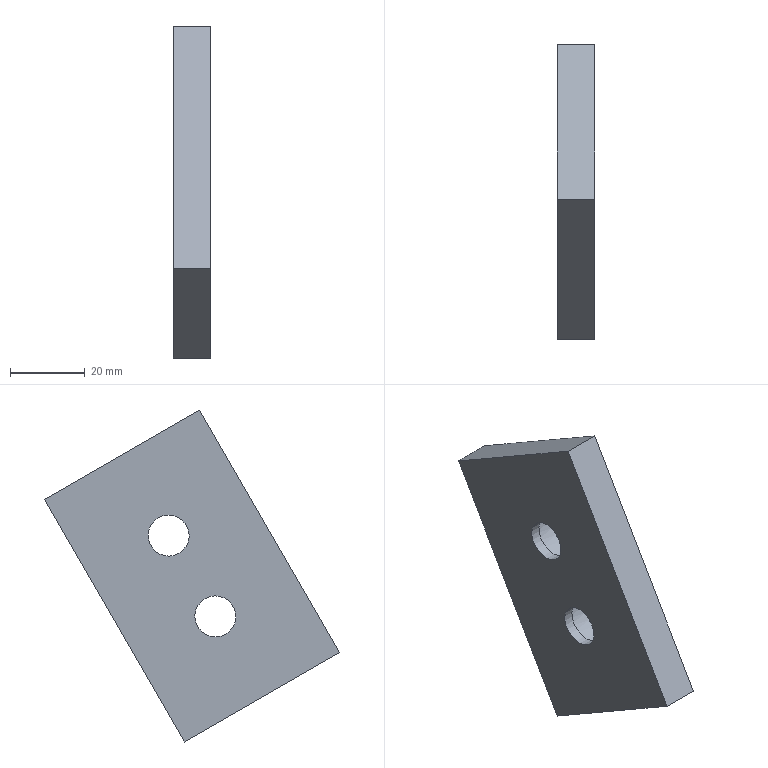Part | NX | features solid 2 | 1 solid | 12 faces | box 10 x 79.069 x 88.952 mm | volume 31975 mm3 | plane 8 | cylinder 4 | commonest cylinder face diameters 11 x2 17.5 x2
STEP:
#1=CARTESIAN_POINT('',(595.,437.58,-241.09));
#2=VERTEX_POINT('',#1);
#3=CARTESIAN_POINT('',(595.,479.149,-265.09));
#4=VERTEX_POINT('',#3);
#5=CARTESIAN_POINT('',(595.,495.17,-274.34));
#6=DIRECTION('',(0.,0.866,-0.5));
#7=VECTOR('',#6,1000.);
#8=LINE('',#5,#7);
#9=EDGE_CURVE('',#2,#4,#8,.T.);
#10=ORIENTED_EDGE('',*,*,#9,.F.);
#11=CARTESIAN_POINT('',(585.,437.58,-241.09));
#12=VERTEX_POINT('',#11);
#13=CARTESIAN_POINT('',(585.,437.58,-241.09));
#14=DIRECTION('',(1.,0.,0.));
#15=VECTOR('',#14,1000.);
#16=LINE('',#13,#15);
#17=EDGE_CURVE('',#12,#2,#16,.T.);
#18=ORIENTED_EDGE('',*,*,#17,.F.);
#19=CARTESIAN_POINT('',(585.,479.149,-265.09));
#20=VERTEX_POINT('',#19);
#21=CARTESIAN_POINT('',(585.,495.17,-274.34));
#22=DIRECTION('',(0.,-0.866,0.5));
#23=VECTOR('',#22,1000.);
#24=LINE('',#21,#23);
#25=EDGE_CURVE('',#12,#20,#24,.F.);
#26=ORIENTED_EDGE('',*,*,#25,.T.);
#27=CARTESIAN_POINT('',(585.,479.149,-265.09));
#28=DIRECTION('',(1.,0.,0.));
#29=VECTOR('',#28,1000.);
#30=LINE('',#27,#29);
#31=EDGE_CURVE('',#20,#4,#30,.T.);
#32=ORIENTED_EDGE('',*,*,#31,.T.);
#33=EDGE_LOOP('',(#10,#18,#26,#32));
#34=FACE_BOUND('',#33,.T.);
#35=CARTESIAN_POINT('',(585.,495.17,-274.34));
#36=DIRECTION('',(0.,0.5,0.866));
#37=DIRECTION('',(1.,0.,0.));
#38=AXIS2_PLACEMENT_3D('',#35,#36,#37);
#39=PLANE('',#38);
#40=ADVANCED_FACE('',(#34),#39,.F.);
#41=CARTESIAN_POINT('',(595.,475.08,-176.138));
#42=VERTEX_POINT('',#41);
#43=CARTESIAN_POINT('',(595.,500.08,-132.837));
#44=DIRECTION('',(0.,-0.5,-0.866));
#45=VECTOR('',#44,1000.);
#46=LINE('',#43,#45);
#47=EDGE_CURVE('',#42,#2,#46,.T.);
#48=ORIENTED_EDGE('',*,*,#47,.F.);
#49=CARTESIAN_POINT('',(585.,475.08,-176.138));
#50=VERTEX_POINT('',#49);
#51=CARTESIAN_POINT('',(585.,475.08,-176.138));
#52=DIRECTION('',(1.,0.,0.));
#53=VECTOR('',#52,1000.);
#54=LINE('',#51,#53);
#55=EDGE_CURVE('',#50,#42,#54,.T.);
#56=ORIENTED_EDGE('',*,*,#55,.F.);
#57=CARTESIAN_POINT('',(585.,462.58,-197.788));
#58=DIRECTION('',(0.,-0.5,-0.866));
#59=VECTOR('',#58,1000.);
#60=LINE('',#57,#59);
#61=EDGE_CURVE('',#50,#12,#60,.T.);
#62=ORIENTED_EDGE('',*,*,#61,.T.);
#63=ORIENTED_EDGE('',*,*,#17,.T.);
#64=EDGE_LOOP('',(#48,#56,#62,#63));
#65=FACE_BOUND('',#64,.T.);
#66=CARTESIAN_POINT('',(585.,462.58,-197.788));
#67=DIRECTION('',(0.,0.866,-0.5));
#68=DIRECTION('',(-1.,0.,0.));
#69=AXIS2_PLACEMENT_3D('',#66,#67,#68);
#70=PLANE('',#69);
#71=ADVANCED_FACE('',(#65),#70,.F.);
#72=CARTESIAN_POINT('',(595.,516.649,-200.138));
#73=VERTEX_POINT('',#72);
#74=CARTESIAN_POINT('',(595.,482.441,-180.388));
#75=DIRECTION('',(0.,-0.866,0.5));
#76=VECTOR('',#75,1000.);
#77=LINE('',#74,#76);
#78=EDGE_CURVE('',#73,#42,#77,.T.);
#79=ORIENTED_EDGE('',*,*,#78,.F.);
#80=CARTESIAN_POINT('',(585.,516.649,-200.138));
#81=VERTEX_POINT('',#80);
#82=CARTESIAN_POINT('',(585.,516.649,-200.138));
#83=DIRECTION('',(1.,0.,0.));
#84=VECTOR('',#83,1000.);
#85=LINE('',#82,#84);
#86=EDGE_CURVE('',#81,#73,#85,.T.);
#87=ORIENTED_EDGE('',*,*,#86,.F.);
#88=CARTESIAN_POINT('',(585.,482.441,-180.388));
#89=DIRECTION('',(0.,0.866,-0.5));
#90=VECTOR('',#89,1000.);
#91=LINE('',#88,#90);
#92=EDGE_CURVE('',#81,#50,#91,.F.);
#93=ORIENTED_EDGE('',*,*,#92,.T.);
#94=ORIENTED_EDGE('',*,*,#55,.T.);
#95=EDGE_LOOP('',(#79,#87,#93,#94));
#96=FACE_BOUND('',#95,.T.);
#97=CARTESIAN_POINT('',(585.,482.441,-180.388));
#98=DIRECTION('',(0.,-0.5,-0.866));
#99=DIRECTION('',(-1.,0.,0.));
#100=AXIS2_PLACEMENT_3D('',#97,#98,#99);
#101=PLANE('',#100);
#102=ADVANCED_FACE('',(#96),#101,.F.);
#103=CARTESIAN_POINT('',(595.,541.649,-156.837));
#104=DIRECTION('',(0.,0.5,0.866));
#105=VECTOR('',#104,1000.);
#106=LINE('',#103,#105);
#107=EDGE_CURVE('',#4,#73,#106,.T.);
#108=ORIENTED_EDGE('',*,*,#107,.F.);
#109=ORIENTED_EDGE('',*,*,#31,.F.);
#110=CARTESIAN_POINT('',(585.,579.149,-91.885));
#111=DIRECTION('',(0.,0.5,0.866));
#112=VECTOR('',#111,1000.);
#113=LINE('',#110,#112);
#114=EDGE_CURVE('',#20,#81,#113,.T.);
#115=ORIENTED_EDGE('',*,*,#114,.T.);
#116=ORIENTED_EDGE('',*,*,#86,.T.);
#117=EDGE_LOOP('',(#108,#109,#115,#116));
#118=FACE_BOUND('',#117,.T.);
#119=CARTESIAN_POINT('',(585.,579.149,-91.885));
#120=DIRECTION('',(0.,-0.866,0.5));
#121=DIRECTION('',(0.,0.5,0.866));
#122=AXIS2_PLACEMENT_3D('',#119,#120,#121);
#123=PLANE('',#122);
#124=ADVANCED_FACE('',(#118),#123,.F.);
#125=CARTESIAN_POINT('',(587.7,475.239,-223.861));
#126=VERTEX_POINT('',#125);
#127=CARTESIAN_POINT('',(587.7,470.864,-231.439));
#128=DIRECTION('',(-1.,0.,0.));
#129=DIRECTION('',(0.,0.5,0.866));
#130=AXIS2_PLACEMENT_3D('',#127,#128,#129);
#131=CIRCLE('',#130,8.75);
#132=EDGE_CURVE('',#126,#126,#131,.T.);
#133=ORIENTED_EDGE('',*,*,#132,.T.);
#134=EDGE_LOOP('',(#133));
#135=FACE_BOUND('',#134,.T.);
#136=CARTESIAN_POINT('',(595.,478.442,-235.814));
#137=VERTEX_POINT('',#136);
#138=CARTESIAN_POINT('',(595.,470.864,-231.439));
#139=DIRECTION('',(1.,0.,0.));
#140=DIRECTION('',(0.,0.866,-0.5));
#141=AXIS2_PLACEMENT_3D('',#138,#139,#140);
#142=CIRCLE('',#141,8.75);
#143=EDGE_CURVE('',#137,#137,#142,.F.);
#144=ORIENTED_EDGE('',*,*,#143,.F.);
#145=EDGE_LOOP('',(#144));
#146=FACE_BOUND('',#145,.T.);
#147=CARTESIAN_POINT('',(605.,470.864,-231.439));
#148=DIRECTION('',(-1.,0.,0.));
#149=DIRECTION('',(0.,0.5,0.866));
#150=AXIS2_PLACEMENT_3D('',#147,#148,#149);
#151=CYLINDRICAL_SURFACE('',#150,8.75);
#152=ADVANCED_FACE('',(#135,#146),#151,.F.);
#153=CARTESIAN_POINT('',(587.7,487.739,-202.211));
#154=VERTEX_POINT('',#153);
#155=CARTESIAN_POINT('',(587.7,483.364,-209.788));
#156=DIRECTION('',(-1.,0.,0.));
#157=DIRECTION('',(0.,0.5,0.866));
#158=AXIS2_PLACEMENT_3D('',#155,#156,#157);
#159=CIRCLE('',#158,8.75);
#160=EDGE_CURVE('',#154,#154,#159,.T.);
#161=ORIENTED_EDGE('',*,*,#160,.T.);
#162=EDGE_LOOP('',(#161));
#163=FACE_BOUND('',#162,.T.);
#164=CARTESIAN_POINT('',(595.,490.942,-214.163));
#165=VERTEX_POINT('',#164);
#166=CARTESIAN_POINT('',(595.,483.364,-209.788));
#167=DIRECTION('',(1.,0.,0.));
#168=DIRECTION('',(0.,0.866,-0.5));
#169=AXIS2_PLACEMENT_3D('',#166,#167,#168);
#170=CIRCLE('',#169,8.75);
#171=EDGE_CURVE('',#165,#165,#170,.F.);
#172=ORIENTED_EDGE('',*,*,#171,.F.);
#173=EDGE_LOOP('',(#172));
#174=FACE_BOUND('',#173,.T.);
#175=CARTESIAN_POINT('',(605.,483.364,-209.788));
#176=DIRECTION('',(-1.,0.,0.));
#177=DIRECTION('',(0.,0.5,0.866));
#178=AXIS2_PLACEMENT_3D('',#175,#176,#177);
#179=CYLINDRICAL_SURFACE('',#178,8.75);
#180=ADVANCED_FACE('',(#163,#174),#179,.F.);
#181=CARTESIAN_POINT('',(585.,486.114,-205.025));
#182=VERTEX_POINT('',#181);
#183=CARTESIAN_POINT('',(585.,483.364,-209.788));
#184=DIRECTION('',(-1.,0.,0.));
#185=DIRECTION('',(0.,0.5,0.866));
#186=AXIS2_PLACEMENT_3D('',#183,#184,#185);
#187=CIRCLE('',#186,5.5);
#188=EDGE_CURVE('',#182,#182,#187,.T.);
#189=ORIENTED_EDGE('',*,*,#188,.F.);
#190=EDGE_LOOP('',(#189));
#191=FACE_BOUND('',#190,.T.);
#192=CARTESIAN_POINT('',(585.,473.614,-226.676));
#193=VERTEX_POINT('',#192);
#194=CARTESIAN_POINT('',(585.,470.864,-231.439));
#195=DIRECTION('',(-1.,0.,0.));
#196=DIRECTION('',(0.,0.5,0.866));
#197=AXIS2_PLACEMENT_3D('',#194,#195,#196);
#198=CIRCLE('',#197,5.5);
#199=EDGE_CURVE('',#193,#193,#198,.T.);
#200=ORIENTED_EDGE('',*,*,#199,.F.);
#201=EDGE_LOOP('',(#200));
#202=FACE_BOUND('',#201,.T.);
#203=ORIENTED_EDGE('',*,*,#92,.F.);
#204=ORIENTED_EDGE('',*,*,#114,.F.);
#205=ORIENTED_EDGE('',*,*,#25,.F.);
#206=ORIENTED_EDGE('',*,*,#61,.F.);
#207=EDGE_LOOP('',(#203,#204,#205,#206));
#208=FACE_BOUND('',#207,.T.);
#209=CARTESIAN_POINT('',(585.,469.941,-202.038));
#210=DIRECTION('',(-1.,0.,0.));
#211=DIRECTION('',(0.,0.5,0.866));
#212=AXIS2_PLACEMENT_3D('',#209,#210,#211);
#213=PLANE('',#212);
#214=ADVANCED_FACE('',(#191,#202,#208),#213,.T.);
#215=ORIENTED_EDGE('',*,*,#199,.T.);
#216=EDGE_LOOP('',(#215));
#217=FACE_BOUND('',#216,.T.);
#218=CARTESIAN_POINT('',(587.7,473.614,-226.676));
#219=VERTEX_POINT('',#218);
#220=CARTESIAN_POINT('',(587.7,470.864,-231.439));
#221=DIRECTION('',(-1.,0.,0.));
#222=DIRECTION('',(0.,0.5,0.866));
#223=AXIS2_PLACEMENT_3D('',#220,#221,#222);
#224=CIRCLE('',#223,5.5);
#225=EDGE_CURVE('',#219,#219,#224,.T.);
#226=ORIENTED_EDGE('',*,*,#225,.F.);
#227=EDGE_LOOP('',(#226));
#228=FACE_BOUND('',#227,.T.);
#229=CARTESIAN_POINT('',(555.,470.864,-231.439));
#230=DIRECTION('',(-1.,0.,0.));
#231=DIRECTION('',(0.,0.5,0.866));
#232=AXIS2_PLACEMENT_3D('',#229,#230,#231);
#233=CYLINDRICAL_SURFACE('',#232,5.5);
#234=ADVANCED_FACE('',(#217,#228),#233,.F.);
#235=ORIENTED_EDGE('',*,*,#225,.T.);
#236=EDGE_LOOP('',(#235));
#237=FACE_BOUND('',#236,.T.);
#238=ORIENTED_EDGE('',*,*,#132,.F.);
#239=EDGE_LOOP('',(#238));
#240=FACE_BOUND('',#239,.T.);
#241=CARTESIAN_POINT('',(587.7,470.864,-231.439));
#242=DIRECTION('',(-1.,0.,0.));
#243=DIRECTION('',(0.,0.5,0.866));
#244=AXIS2_PLACEMENT_3D('',#241,#242,#243);
#245=PLANE('',#244);
#246=ADVANCED_FACE('',(#237,#240),#245,.F.);
#247=ORIENTED_EDGE('',*,*,#188,.T.);
#248=EDGE_LOOP('',(#247));
#249=FACE_BOUND('',#248,.T.);
#250=CARTESIAN_POINT('',(587.7,486.114,-205.025));
#251=VERTEX_POINT('',#250);
#252=CARTESIAN_POINT('',(587.7,483.364,-209.788));
#253=DIRECTION('',(-1.,0.,0.));
#254=DIRECTION('',(0.,0.5,0.866));
#255=AXIS2_PLACEMENT_3D('',#252,#253,#254);
#256=CIRCLE('',#255,5.5);
#257=EDGE_CURVE('',#251,#251,#256,.T.);
#258=ORIENTED_EDGE('',*,*,#257,.F.);
#259=EDGE_LOOP('',(#258));
#260=FACE_BOUND('',#259,.T.);
#261=CARTESIAN_POINT('',(555.,483.364,-209.788));
#262=DIRECTION('',(-1.,0.,0.));
#263=DIRECTION('',(0.,0.5,0.866));
#264=AXIS2_PLACEMENT_3D('',#261,#262,#263);
#265=CYLINDRICAL_SURFACE('',#264,5.5);
#266=ADVANCED_FACE('',(#249,#260),#265,.F.);
#267=ORIENTED_EDGE('',*,*,#257,.T.);
#268=EDGE_LOOP('',(#267));
#269=FACE_BOUND('',#268,.T.);
#270=ORIENTED_EDGE('',*,*,#160,.F.);
#271=EDGE_LOOP('',(#270));
#272=FACE_BOUND('',#271,.T.);
#273=CARTESIAN_POINT('',(587.7,483.364,-209.788));
#274=DIRECTION('',(-1.,0.,0.));
#275=DIRECTION('',(0.,0.5,0.866));
#276=AXIS2_PLACEMENT_3D('',#273,#274,#275);
#277=PLANE('',#276);
#278=ADVANCED_FACE('',(#269,#272),#277,.F.);
#279=ORIENTED_EDGE('',*,*,#143,.T.);
#280=EDGE_LOOP('',(#279));
#281=FACE_BOUND('',#280,.T.);
#282=ORIENTED_EDGE('',*,*,#171,.T.);
#283=EDGE_LOOP('',(#282));
#284=FACE_BOUND('',#283,.T.);
#285=ORIENTED_EDGE('',*,*,#47,.T.);
#286=ORIENTED_EDGE('',*,*,#9,.T.);
#287=ORIENTED_EDGE('',*,*,#107,.T.);
#288=ORIENTED_EDGE('',*,*,#78,.T.);
#289=EDGE_LOOP('',(#285,#286,#287,#288));
#290=FACE_BOUND('',#289,.T.);
#291=CARTESIAN_POINT('',(595.,532.556,-151.587));
#292=DIRECTION('',(1.,0.,0.));
#293=DIRECTION('',(0.,0.866,-0.5));
#294=AXIS2_PLACEMENT_3D('',#291,#292,#293);
#295=PLANE('',#294);
#296=ADVANCED_FACE('',(#281,#284,#290),#295,.T.);
#297=CLOSED_SHELL('',(#40,#71,#102,#124,#152,#180,#214,#234,#246,#266,#278,#296));
#298=MANIFOLD_SOLID_BREP('',#297);
#299=(LENGTH_UNIT()NAMED_UNIT(*)SI_UNIT(.MILLI.,.METRE.));
#300=UNCERTAINTY_MEASURE_WITH_UNIT(LENGTH_MEASURE(0.00001),#299,'','');
#301=(NAMED_UNIT(*)PLANE_ANGLE_UNIT()SI_UNIT($,.RADIAN.));
#302=(NAMED_UNIT(*)SI_UNIT($,.STERADIAN.)SOLID_ANGLE_UNIT());
#303=(GEOMETRIC_REPRESENTATION_CONTEXT(3)GLOBAL_UNCERTAINTY_ASSIGNED_CONTEXT((#300))GLOBAL_UNIT_ASSIGNED_CONTEXT((#299,#301,#302))REPRESENTATION_CONTEXT('',''));
#304=ADVANCED_BREP_SHAPE_REPRESENTATION('',(#298),#303);